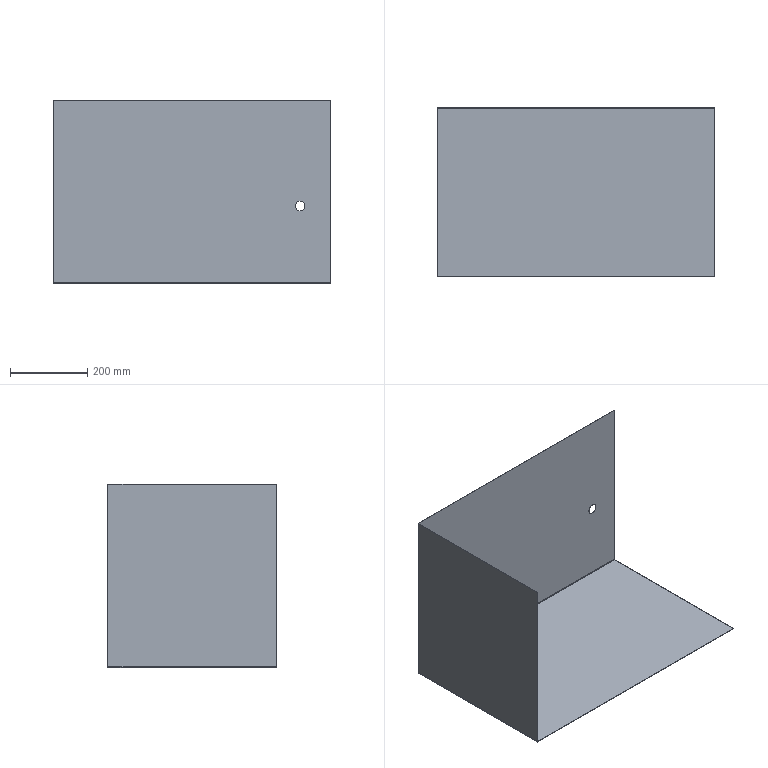Part | 1 solid | 24 faces | box 721 x 440 x 475 mm | volume 1037227 mm3 | plane 16 | cylinder 6 | spline 2 | commonest cylinder face diameters 1.473 x2 3.873 x2 25 x2
STEP:
#1=CARTESIAN_POINT('',(280.5,220.,212.5));
#2=VERTEX_POINT('',#1);
#3=CARTESIAN_POINT('',(280.5,220.,187.5));
#4=VERTEX_POINT('',#3);
#5=CARTESIAN_POINT('',(280.5,220.,200.));
#6=DIRECTION('',(0.,-1.,0.));
#7=DIRECTION('',(0.,0.,-1.));
#8=AXIS2_PLACEMENT_3D('',#5,#6,#7);
#9=CIRCLE('',#8,12.5);
#10=EDGE_CURVE('',#2,#4,#9,.T.);
#11=ORIENTED_EDGE('',*,*,#10,.F.);
#12=CARTESIAN_POINT('',(280.5,218.8,212.5));
#13=VERTEX_POINT('',#12);
#14=CARTESIAN_POINT('',(280.5,220.,212.5));
#15=DIRECTION('',(0.,-1.,0.));
#16=VECTOR('',#15,1000.);
#17=LINE('',#14,#16);
#18=EDGE_CURVE('',#2,#13,#17,.T.);
#19=ORIENTED_EDGE('',*,*,#18,.T.);
#20=CARTESIAN_POINT('',(280.5,218.8,187.5));
#21=VERTEX_POINT('',#20);
#22=CARTESIAN_POINT('',(280.5,218.8,200.));
#23=DIRECTION('',(0.,-1.,0.));
#24=DIRECTION('',(0.,0.,-1.));
#25=AXIS2_PLACEMENT_3D('',#22,#23,#24);
#26=CIRCLE('',#25,12.5);
#27=EDGE_CURVE('',#13,#21,#26,.T.);
#28=ORIENTED_EDGE('',*,*,#27,.T.);
#29=CARTESIAN_POINT('',(280.5,220.,187.5));
#30=DIRECTION('',(0.,-1.,0.));
#31=VECTOR('',#30,1000.);
#32=LINE('',#29,#31);
#33=EDGE_CURVE('',#4,#21,#32,.T.);
#34=ORIENTED_EDGE('',*,*,#33,.F.);
#35=EDGE_LOOP('',(#11,#19,#28,#34));
#36=FACE_OUTER_BOUND('',#35,.T.);
#37=CARTESIAN_POINT('',(280.5,220.,200.));
#38=DIRECTION('',(0.,-1.,0.));
#39=DIRECTION('',(0.,0.,-1.));
#40=AXIS2_PLACEMENT_3D('',#37,#38,#39);
#41=CYLINDRICAL_SURFACE('',#40,12.5);
#42=ADVANCED_FACE('',(#36),#41,.F.);
#43=CARTESIAN_POINT('',(-358.563,-220.,-1.2));
#44=VERTEX_POINT('',#43);
#45=CARTESIAN_POINT('',(-358.563,218.063,-1.2));
#46=VERTEX_POINT('',#45);
#47=CARTESIAN_POINT('',(-358.563,-220.,-1.2));
#48=DIRECTION('',(0.,1.,0.));
#49=VECTOR('',#48,1000.);
#50=LINE('',#47,#49);
#51=EDGE_CURVE('',#44,#46,#50,.T.);
#52=ORIENTED_EDGE('',*,*,#51,.T.);
#53=CARTESIAN_POINT('',(360.5,218.063,-1.2));
#54=VERTEX_POINT('',#53);
#55=CARTESIAN_POINT('',(-358.593,218.063,-1.2));
#56=DIRECTION('',(1.,0.,0.));
#57=VECTOR('',#56,1000.);
#58=LINE('',#55,#57);
#59=EDGE_CURVE('',#46,#54,#58,.T.);
#60=ORIENTED_EDGE('',*,*,#59,.T.);
#61=CARTESIAN_POINT('',(360.5,-220.,-1.2));
#62=VERTEX_POINT('',#61);
#63=CARTESIAN_POINT('',(360.5,220.,-1.2));
#64=DIRECTION('',(0.,1.,0.));
#65=VECTOR('',#64,1000.);
#66=LINE('',#63,#65);
#67=EDGE_CURVE('',#62,#54,#66,.T.);
#68=ORIENTED_EDGE('',*,*,#67,.F.);
#69=CARTESIAN_POINT('',(-360.5,-220.,-1.2));
#70=DIRECTION('',(1.,0.,0.));
#71=VECTOR('',#70,1000.);
#72=LINE('',#69,#71);
#73=EDGE_CURVE('',#44,#62,#72,.T.);
#74=ORIENTED_EDGE('',*,*,#73,.F.);
#75=EDGE_LOOP('',(#52,#60,#68,#74));
#76=FACE_OUTER_BOUND('',#75,.T.);
#77=CARTESIAN_POINT('',(0.,0.,-1.2));
#78=DIRECTION('',(0.,0.,1.));
#79=DIRECTION('',(1.,0.,0.));
#80=AXIS2_PLACEMENT_3D('',#77,#78,#79);
#81=PLANE('',#80);
#82=ADVANCED_FACE('',(#76),#81,.F.);
#83=CARTESIAN_POINT('',(-358.563,218.063,0.));
#84=VERTEX_POINT('',#83);
#85=CARTESIAN_POINT('',(360.5,218.063,0.));
#86=VERTEX_POINT('',#85);
#87=CARTESIAN_POINT('',(-358.593,218.063,0.));
#88=DIRECTION('',(1.,0.,0.));
#89=VECTOR('',#88,1000.);
#90=LINE('',#87,#89);
#91=EDGE_CURVE('',#84,#86,#90,.T.);
#92=ORIENTED_EDGE('',*,*,#91,.F.);
#93=CARTESIAN_POINT('',(-358.563,-220.,0.));
#94=VERTEX_POINT('',#93);
#95=CARTESIAN_POINT('',(-358.563,-220.,0.));
#96=DIRECTION('',(0.,1.,0.));
#97=VECTOR('',#96,1000.);
#98=LINE('',#95,#97);
#99=EDGE_CURVE('',#94,#84,#98,.T.);
#100=ORIENTED_EDGE('',*,*,#99,.F.);
#101=CARTESIAN_POINT('',(360.5,-220.,0.));
#102=VERTEX_POINT('',#101);
#103=CARTESIAN_POINT('',(-360.5,-220.,0.));
#104=DIRECTION('',(1.,0.,0.));
#105=VECTOR('',#104,1000.);
#106=LINE('',#103,#105);
#107=EDGE_CURVE('',#94,#102,#106,.T.);
#108=ORIENTED_EDGE('',*,*,#107,.T.);
#109=CARTESIAN_POINT('',(360.5,220.,0.));
#110=DIRECTION('',(0.,1.,0.));
#111=VECTOR('',#110,1000.);
#112=LINE('',#109,#111);
#113=EDGE_CURVE('',#102,#86,#112,.T.);
#114=ORIENTED_EDGE('',*,*,#113,.T.);
#115=EDGE_LOOP('',(#92,#100,#108,#114));
#116=FACE_OUTER_BOUND('',#115,.T.);
#117=CARTESIAN_POINT('',(0.,0.,0.));
#118=DIRECTION('',(0.,0.,1.));
#119=DIRECTION('',(1.,0.,0.));
#120=AXIS2_PLACEMENT_3D('',#117,#118,#119);
#121=PLANE('',#120);
#122=ADVANCED_FACE('',(#116),#121,.T.);
#123=ORIENTED_EDGE('',*,*,#107,.F.);
#124=CARTESIAN_POINT('',(-358.563,-220.,0.));
#125=DIRECTION('',(0.,0.,-1.));
#126=VECTOR('',#125,1000.);
#127=LINE('',#124,#126);
#128=EDGE_CURVE('',#94,#44,#127,.T.);
#129=ORIENTED_EDGE('',*,*,#128,.T.);
#130=ORIENTED_EDGE('',*,*,#73,.T.);
#131=CARTESIAN_POINT('',(360.5,-220.,-1.2));
#132=DIRECTION('',(0.,0.,1.));
#133=VECTOR('',#132,1000.);
#134=LINE('',#131,#133);
#135=EDGE_CURVE('',#62,#102,#134,.T.);
#136=ORIENTED_EDGE('',*,*,#135,.T.);
#137=EDGE_LOOP('',(#123,#129,#130,#136));
#138=FACE_OUTER_BOUND('',#137,.T.);
#139=CARTESIAN_POINT('',(-360.5,-220.,-1.2));
#140=DIRECTION('',(0.,-1.,0.));
#141=DIRECTION('',(0.,0.,-1.));
#142=AXIS2_PLACEMENT_3D('',#139,#140,#141);
#143=PLANE('',#142);
#144=ADVANCED_FACE('',(#138),#143,.T.);
#145=CARTESIAN_POINT('',(360.5,218.063,0.));
#146=DIRECTION('',(0.,0.,-1.));
#147=VECTOR('',#146,1000.);
#148=LINE('',#145,#147);
#149=EDGE_CURVE('',#86,#54,#148,.T.);
#150=ORIENTED_EDGE('',*,*,#149,.F.);
#151=ORIENTED_EDGE('',*,*,#113,.F.);
#152=ORIENTED_EDGE('',*,*,#135,.F.);
#153=ORIENTED_EDGE('',*,*,#67,.T.);
#154=EDGE_LOOP('',(#150,#151,#152,#153));
#155=FACE_OUTER_BOUND('',#154,.T.);
#156=CARTESIAN_POINT('',(360.5,220.,-1.2));
#157=DIRECTION('',(1.,0.,0.));
#158=DIRECTION('',(0.,1.,0.));
#159=AXIS2_PLACEMENT_3D('',#156,#157,#158);
#160=PLANE('',#159);
#161=ADVANCED_FACE('',(#155),#160,.T.);
#162=CARTESIAN_POINT('',(360.5,218.8,0.7366));
#163=VERTEX_POINT('',#162);
#164=CARTESIAN_POINT('',(360.5,220.,0.7366));
#165=VERTEX_POINT('',#164);
#166=CARTESIAN_POINT('',(360.5,220.,0.7366));
#167=DIRECTION('',(0.,1.,0.));
#168=VECTOR('',#167,1000.);
#169=LINE('',#166,#168);
#170=EDGE_CURVE('',#163,#165,#169,.T.);
#171=ORIENTED_EDGE('',*,*,#170,.F.);
#172=CARTESIAN_POINT('',(360.5,218.063,0.7366));
#173=DIRECTION('',(1.,0.,0.));
#174=DIRECTION('',(0.,0.,1.));
#175=AXIS2_PLACEMENT_3D('',#172,#173,#174);
#176=CIRCLE('',#175,0.7366);
#177=EDGE_CURVE('',#86,#163,#176,.T.);
#178=ORIENTED_EDGE('',*,*,#177,.F.);
#179=ORIENTED_EDGE('',*,*,#149,.T.);
#180=CARTESIAN_POINT('',(360.5,218.063,0.7366));
#181=DIRECTION('',(1.,0.,0.));
#182=DIRECTION('',(0.,0.,1.));
#183=AXIS2_PLACEMENT_3D('',#180,#181,#182);
#184=CIRCLE('',#183,1.937);
#185=EDGE_CURVE('',#54,#165,#184,.T.);
#186=ORIENTED_EDGE('',*,*,#185,.T.);
#187=EDGE_LOOP('',(#171,#178,#179,#186));
#188=FACE_OUTER_BOUND('',#187,.T.);
#189=CARTESIAN_POINT('',(360.5,218.063,0.7366));
#190=DIRECTION('',(1.,0.,0.));
#191=DIRECTION('',(0.,0.,-1.));
#192=AXIS2_PLACEMENT_3D('',#189,#190,#191);
#193=PLANE('',#192);
#194=ADVANCED_FACE('',(#188),#193,.T.);
#195=CARTESIAN_POINT('',(-358.593,218.8,0.7366));
#196=VERTEX_POINT('',#195);
#197=CARTESIAN_POINT('',(-358.593,218.8,0.7366));
#198=CARTESIAN_POINT('',(-358.588,218.8,0.5438));
#199=CARTESIAN_POINT('',(-358.583,218.721,0.3521));
#200=CARTESIAN_POINT('',(-358.573,218.448,0.07939));
#201=CARTESIAN_POINT('',(-358.568,218.256,0.));
#202=CARTESIAN_POINT('',(-358.563,218.063,0.));
#203=B_SPLINE_CURVE_WITH_KNOTS('',3,(#197,#198,#199,#200,#201,#202),.UNSPECIFIED.,.F.,.F.,(4,2,4),(0.,0.5,1.),.UNSPECIFIED.);
#204=EDGE_CURVE('',#196,#84,#203,.T.);
#205=ORIENTED_EDGE('',*,*,#204,.F.);
#206=CARTESIAN_POINT('',(-358.593,220.,0.7366));
#207=VERTEX_POINT('',#206);
#208=CARTESIAN_POINT('',(-358.593,218.8,0.7366));
#209=DIRECTION('',(0.,-1.,0.));
#210=VECTOR('',#209,1000.);
#211=LINE('',#208,#210);
#212=EDGE_CURVE('',#207,#196,#211,.T.);
#213=ORIENTED_EDGE('',*,*,#212,.F.);
#214=CARTESIAN_POINT('',(-358.593,220.,0.7366));
#215=CARTESIAN_POINT('',(-358.59,220.,0.4831));
#216=CARTESIAN_POINT('',(-358.588,219.95,0.2297));
#217=CARTESIAN_POINT('',(-358.583,219.756,-0.2387));
#218=CARTESIAN_POINT('',(-358.581,219.612,-0.4535));
#219=CARTESIAN_POINT('',(-358.576,219.254,-0.812));
#220=CARTESIAN_POINT('',(-358.573,219.039,-0.9556));
#221=CARTESIAN_POINT('',(-358.568,218.57,-1.15));
#222=CARTESIAN_POINT('',(-358.566,218.317,-1.2));
#223=CARTESIAN_POINT('',(-358.563,218.063,-1.2));
#224=B_SPLINE_CURVE_WITH_KNOTS('',3,(#214,#215,#216,#217,#218,#219,#220,#221,#222,#223),.UNSPECIFIED.,.F.,.F.,(4,2,2,2,4),(0.,0.25,0.5,0.75,1.),.UNSPECIFIED.);
#225=EDGE_CURVE('',#207,#46,#224,.T.);
#226=ORIENTED_EDGE('',*,*,#225,.T.);
#227=CARTESIAN_POINT('',(-358.563,218.063,0.));
#228=DIRECTION('',(0.,0.,-1.));
#229=VECTOR('',#228,1000.);
#230=LINE('',#227,#229);
#231=EDGE_CURVE('',#84,#46,#230,.T.);
#232=ORIENTED_EDGE('',*,*,#231,.F.);
#233=EDGE_LOOP('',(#205,#213,#226,#232));
#234=FACE_OUTER_BOUND('',#233,.T.);
#235=CARTESIAN_POINT('',(-358.593,220.012,0.7366));
#236=CARTESIAN_POINT('',(-358.59,220.012,0.4815));
#237=CARTESIAN_POINT('',(-358.588,219.961,0.2266));
#238=CARTESIAN_POINT('',(-358.583,219.766,-0.2448));
#239=CARTESIAN_POINT('',(-358.581,219.622,-0.4609));
#240=CARTESIAN_POINT('',(-358.576,219.261,-0.8216));
#241=CARTESIAN_POINT('',(-358.573,219.045,-0.9661));
#242=CARTESIAN_POINT('',(-358.568,218.573,-1.161));
#243=CARTESIAN_POINT('',(-358.566,218.319,-1.212));
#244=CARTESIAN_POINT('',(-358.563,218.063,-1.212));
#245=CARTESIAN_POINT('',(-358.593,220.,0.7366));
#246=CARTESIAN_POINT('',(-358.59,220.,0.4831));
#247=CARTESIAN_POINT('',(-358.588,219.95,0.2297));
#248=CARTESIAN_POINT('',(-358.583,219.756,-0.2387));
#249=CARTESIAN_POINT('',(-358.581,219.612,-0.4535));
#250=CARTESIAN_POINT('',(-358.576,219.254,-0.812));
#251=CARTESIAN_POINT('',(-358.573,219.039,-0.9556));
#252=CARTESIAN_POINT('',(-358.568,218.57,-1.15));
#253=CARTESIAN_POINT('',(-358.566,218.317,-1.2));
#254=CARTESIAN_POINT('',(-358.563,218.063,-1.2));
#255=CARTESIAN_POINT('',(-358.593,218.8,0.7366));
#256=CARTESIAN_POINT('',(-358.59,218.8,0.6402));
#257=CARTESIAN_POINT('',(-358.588,218.781,0.5438));
#258=CARTESIAN_POINT('',(-358.583,218.707,0.3656));
#259=CARTESIAN_POINT('',(-358.581,218.652,0.2839));
#260=CARTESIAN_POINT('',(-358.576,218.516,0.1476));
#261=CARTESIAN_POINT('',(-358.573,218.434,0.09297));
#262=CARTESIAN_POINT('',(-358.568,218.256,0.01917));
#263=CARTESIAN_POINT('',(-358.566,218.16,0.));
#264=CARTESIAN_POINT('',(-358.563,218.063,0.));
#265=CARTESIAN_POINT('',(-358.593,218.788,0.7366));
#266=CARTESIAN_POINT('',(-358.59,218.788,0.6417));
#267=CARTESIAN_POINT('',(-358.588,218.769,0.547));
#268=CARTESIAN_POINT('',(-358.583,218.696,0.3717));
#269=CARTESIAN_POINT('',(-358.581,218.643,0.2914));
#270=CARTESIAN_POINT('',(-358.576,218.509,0.1573));
#271=CARTESIAN_POINT('',(-358.573,218.428,0.1036));
#272=CARTESIAN_POINT('',(-358.568,218.253,0.03098));
#273=CARTESIAN_POINT('',(-358.566,218.158,0.01212));
#274=CARTESIAN_POINT('',(-358.563,218.063,0.01212));
#275=B_SPLINE_SURFACE_WITH_KNOTS('',1,3,((#235,#236,#237,#238,#239,#240,#241,#242,#243,#244),(#245,#246,#247,#248,#249,#250,#251,#252,#253,#254),(#255,#256,#257,#258,#259,#260,#261,#262,#263,#264),(#265,#266,#267,#268,#269,#270,#271,#272,#273,#274)),.UNSPECIFIED.,.F.,.F.,.F.,(2,1,1,2),(4,2,2,2,4),(-0.01,0.,1.,1.01),(0.,0.25,0.5,0.75,1.),.UNSPECIFIED.);
#276=ADVANCED_FACE('',(#234),#275,.F.);
#277=ORIENTED_EDGE('',*,*,#59,.F.);
#278=ORIENTED_EDGE('',*,*,#225,.F.);
#279=CARTESIAN_POINT('',(0.,220.,0.7366));
#280=DIRECTION('',(-1.,0.,0.));
#281=VECTOR('',#280,1000.);
#282=LINE('',#279,#281);
#283=EDGE_CURVE('',#165,#207,#282,.T.);
#284=ORIENTED_EDGE('',*,*,#283,.F.);
#285=ORIENTED_EDGE('',*,*,#185,.F.);
#286=EDGE_LOOP('',(#277,#278,#284,#285));
#287=FACE_OUTER_BOUND('',#286,.T.);
#288=CARTESIAN_POINT('',(-358.593,218.063,0.7366));
#289=DIRECTION('',(-1.,0.,0.));
#290=DIRECTION('',(0.,1.,0.));
#291=AXIS2_PLACEMENT_3D('',#288,#289,#290);
#292=CYLINDRICAL_SURFACE('',#291,1.937);
#293=ADVANCED_FACE('',(#287),#292,.T.);
#294=ORIENTED_EDGE('',*,*,#91,.T.);
#295=ORIENTED_EDGE('',*,*,#177,.T.);
#296=CARTESIAN_POINT('',(360.5,218.8,0.7366));
#297=DIRECTION('',(-1.,0.,0.));
#298=VECTOR('',#297,1000.);
#299=LINE('',#296,#298);
#300=EDGE_CURVE('',#163,#196,#299,.T.);
#301=ORIENTED_EDGE('',*,*,#300,.T.);
#302=ORIENTED_EDGE('',*,*,#204,.T.);
#303=EDGE_LOOP('',(#294,#295,#301,#302));
#304=FACE_OUTER_BOUND('',#303,.T.);
#305=CARTESIAN_POINT('',(-358.593,218.063,0.7366));
#306=DIRECTION('',(-1.,0.,0.));
#307=DIRECTION('',(0.,1.,0.));
#308=AXIS2_PLACEMENT_3D('',#305,#306,#307);
#309=CYLINDRICAL_SURFACE('',#308,0.7366);
#310=ADVANCED_FACE('',(#304),#309,.F.);
#311=CARTESIAN_POINT('',(360.5,218.8,473.8));
#312=VERTEX_POINT('',#311);
#313=CARTESIAN_POINT('',(360.5,218.8,0.));
#314=DIRECTION('',(0.,0.,1.));
#315=VECTOR('',#314,1000.);
#316=LINE('',#313,#315);
#317=EDGE_CURVE('',#163,#312,#316,.T.);
#318=ORIENTED_EDGE('',*,*,#317,.F.);
#319=ORIENTED_EDGE('',*,*,#170,.T.);
#320=CARTESIAN_POINT('',(360.5,220.,473.8));
#321=VERTEX_POINT('',#320);
#322=CARTESIAN_POINT('',(360.5,220.,473.8));
#323=DIRECTION('',(0.,0.,1.));
#324=VECTOR('',#323,1000.);
#325=LINE('',#322,#324);
#326=EDGE_CURVE('',#165,#321,#325,.T.);
#327=ORIENTED_EDGE('',*,*,#326,.T.);
#328=CARTESIAN_POINT('',(360.5,220.,473.8));
#329=DIRECTION('',(0.,-1.,0.));
#330=VECTOR('',#329,1000.);
#331=LINE('',#328,#330);
#332=EDGE_CURVE('',#321,#312,#331,.T.);
#333=ORIENTED_EDGE('',*,*,#332,.T.);
#334=EDGE_LOOP('',(#318,#319,#327,#333));
#335=FACE_OUTER_BOUND('',#334,.T.);
#336=CARTESIAN_POINT('',(360.5,220.,473.8));
#337=DIRECTION('',(1.,0.,0.));
#338=DIRECTION('',(0.,0.,-1.));
#339=AXIS2_PLACEMENT_3D('',#336,#337,#338);
#340=PLANE('',#339);
#341=ADVANCED_FACE('',(#335),#340,.T.);
#342=CARTESIAN_POINT('',(280.5,220.,200.));
#343=DIRECTION('',(0.,-1.,0.));
#344=DIRECTION('',(0.,0.,-1.));
#345=AXIS2_PLACEMENT_3D('',#342,#343,#344);
#346=CIRCLE('',#345,12.5);
#347=EDGE_CURVE('',#4,#2,#346,.T.);
#348=ORIENTED_EDGE('',*,*,#347,.T.);
#349=ORIENTED_EDGE('',*,*,#10,.T.);
#350=EDGE_LOOP('',(#348,#349));
#351=FACE_BOUND('',#350,.T.);
#352=CARTESIAN_POINT('',(-358.593,220.,473.8));
#353=VERTEX_POINT('',#352);
#354=CARTESIAN_POINT('',(-358.593,220.,0.));
#355=DIRECTION('',(0.,0.,-1.));
#356=VECTOR('',#355,1000.);
#357=LINE('',#354,#356);
#358=EDGE_CURVE('',#353,#207,#357,.T.);
#359=ORIENTED_EDGE('',*,*,#358,.F.);
#360=CARTESIAN_POINT('',(-360.5,220.,473.8));
#361=DIRECTION('',(-1.,0.,0.));
#362=VECTOR('',#361,1000.);
#363=LINE('',#360,#362);
#364=EDGE_CURVE('',#321,#353,#363,.T.);
#365=ORIENTED_EDGE('',*,*,#364,.F.);
#366=ORIENTED_EDGE('',*,*,#326,.F.);
#367=ORIENTED_EDGE('',*,*,#283,.T.);
#368=EDGE_LOOP('',(#359,#365,#366,#367));
#369=FACE_OUTER_BOUND('',#368,.T.);
#370=CARTESIAN_POINT('',(0.,220.,0.));
#371=DIRECTION('',(0.,1.,0.));
#372=DIRECTION('',(0.,0.,1.));
#373=AXIS2_PLACEMENT_3D('',#370,#371,#372);
#374=PLANE('',#373);
#375=ADVANCED_FACE('',(#351,#369),#374,.T.);
#376=CARTESIAN_POINT('',(280.5,218.8,200.));
#377=DIRECTION('',(0.,-1.,0.));
#378=DIRECTION('',(0.,0.,-1.));
#379=AXIS2_PLACEMENT_3D('',#376,#377,#378);
#380=CIRCLE('',#379,12.5);
#381=EDGE_CURVE('',#21,#13,#380,.T.);
#382=ORIENTED_EDGE('',*,*,#381,.F.);
#383=ORIENTED_EDGE('',*,*,#27,.F.);
#384=EDGE_LOOP('',(#382,#383));
#385=FACE_BOUND('',#384,.T.);
#386=CARTESIAN_POINT('',(-358.593,218.8,473.8));
#387=VERTEX_POINT('',#386);
#388=CARTESIAN_POINT('',(0.,218.8,473.8));
#389=DIRECTION('',(-1.,0.,0.));
#390=VECTOR('',#389,1000.);
#391=LINE('',#388,#390);
#392=EDGE_CURVE('',#312,#387,#391,.T.);
#393=ORIENTED_EDGE('',*,*,#392,.T.);
#394=CARTESIAN_POINT('',(-358.593,218.8,0.));
#395=DIRECTION('',(0.,0.,1.));
#396=VECTOR('',#395,1000.);
#397=LINE('',#394,#396);
#398=EDGE_CURVE('',#196,#387,#397,.T.);
#399=ORIENTED_EDGE('',*,*,#398,.F.);
#400=ORIENTED_EDGE('',*,*,#300,.F.);
#401=ORIENTED_EDGE('',*,*,#317,.T.);
#402=EDGE_LOOP('',(#393,#399,#400,#401));
#403=FACE_OUTER_BOUND('',#402,.T.);
#404=CARTESIAN_POINT('',(0.,218.8,0.));
#405=DIRECTION('',(0.,1.,0.));
#406=DIRECTION('',(0.,0.,1.));
#407=AXIS2_PLACEMENT_3D('',#404,#405,#406);
#408=PLANE('',#407);
#409=ADVANCED_FACE('',(#385,#403),#408,.F.);
#410=CARTESIAN_POINT('',(-358.593,218.8,473.8));
#411=DIRECTION('',(0.,1.,0.));
#412=VECTOR('',#411,1000.);
#413=LINE('',#410,#412);
#414=EDGE_CURVE('',#387,#353,#413,.T.);
#415=ORIENTED_EDGE('',*,*,#414,.F.);
#416=ORIENTED_EDGE('',*,*,#392,.F.);
#417=ORIENTED_EDGE('',*,*,#332,.F.);
#418=ORIENTED_EDGE('',*,*,#364,.T.);
#419=EDGE_LOOP('',(#415,#416,#417,#418));
#420=FACE_OUTER_BOUND('',#419,.T.);
#421=CARTESIAN_POINT('',(-360.5,220.,473.8));
#422=DIRECTION('',(0.,0.,1.));
#423=DIRECTION('',(0.,-1.,0.));
#424=AXIS2_PLACEMENT_3D('',#421,#422,#423);
#425=PLANE('',#424);
#426=ADVANCED_FACE('',(#420),#425,.T.);
#427=ORIENTED_EDGE('',*,*,#398,.T.);
#428=ORIENTED_EDGE('',*,*,#414,.T.);
#429=ORIENTED_EDGE('',*,*,#358,.T.);
#430=ORIENTED_EDGE('',*,*,#212,.T.);
#431=EDGE_LOOP('',(#427,#428,#429,#430));
#432=FACE_OUTER_BOUND('',#431,.T.);
#433=CARTESIAN_POINT('',(-358.593,218.8,0.));
#434=DIRECTION('',(1.,0.,0.));
#435=DIRECTION('',(0.,0.,-1.));
#436=AXIS2_PLACEMENT_3D('',#433,#434,#435);
#437=PLANE('',#436);
#438=ADVANCED_FACE('',(#432),#437,.F.);
#439=CARTESIAN_POINT('',(-360.5,218.093,0.7366));
#440=VERTEX_POINT('',#439);
#441=CARTESIAN_POINT('',(-359.3,218.093,0.7366));
#442=VERTEX_POINT('',#441);
#443=CARTESIAN_POINT('',(-359.3,218.093,0.7366));
#444=DIRECTION('',(1.,0.,0.));
#445=VECTOR('',#444,1000.);
#446=LINE('',#443,#445);
#447=EDGE_CURVE('',#440,#442,#446,.T.);
#448=ORIENTED_EDGE('',*,*,#447,.T.);
#449=CARTESIAN_POINT('',(-358.563,218.063,0.));
#450=CARTESIAN_POINT('',(-358.756,218.068,0.));
#451=CARTESIAN_POINT('',(-358.948,218.073,0.07939));
#452=CARTESIAN_POINT('',(-359.221,218.083,0.3521));
#453=CARTESIAN_POINT('',(-359.3,218.088,0.5438));
#454=CARTESIAN_POINT('',(-359.3,218.093,0.7366));
#455=B_SPLINE_CURVE_WITH_KNOTS('',3,(#449,#450,#451,#452,#453,#454),.UNSPECIFIED.,.F.,.F.,(4,2,4),(0.,0.5,1.),.UNSPECIFIED.);
#456=EDGE_CURVE('',#84,#442,#455,.T.);
#457=ORIENTED_EDGE('',*,*,#456,.F.);
#458=ORIENTED_EDGE('',*,*,#231,.T.);
#459=CARTESIAN_POINT('',(-358.563,218.063,-1.2));
#460=CARTESIAN_POINT('',(-358.817,218.066,-1.2));
#461=CARTESIAN_POINT('',(-359.07,218.068,-1.15));
#462=CARTESIAN_POINT('',(-359.539,218.073,-0.9556));
#463=CARTESIAN_POINT('',(-359.754,218.076,-0.812));
#464=CARTESIAN_POINT('',(-360.112,218.081,-0.4535));
#465=CARTESIAN_POINT('',(-360.256,218.083,-0.2387));
#466=CARTESIAN_POINT('',(-360.45,218.088,0.2297));
#467=CARTESIAN_POINT('',(-360.5,218.09,0.4831));
#468=CARTESIAN_POINT('',(-360.5,218.093,0.7366));
#469=B_SPLINE_CURVE_WITH_KNOTS('',3,(#459,#460,#461,#462,#463,#464,#465,#466,#467,#468),.UNSPECIFIED.,.F.,.F.,(4,2,2,2,4),(0.,0.25,0.5,0.75,1.),.UNSPECIFIED.);
#470=EDGE_CURVE('',#46,#440,#469,.T.);
#471=ORIENTED_EDGE('',*,*,#470,.T.);
#472=EDGE_LOOP('',(#448,#457,#458,#471));
#473=FACE_OUTER_BOUND('',#472,.T.);
#474=CARTESIAN_POINT('',(-358.563,218.063,-1.212));
#475=CARTESIAN_POINT('',(-358.819,218.066,-1.212));
#476=CARTESIAN_POINT('',(-359.073,218.068,-1.161));
#477=CARTESIAN_POINT('',(-359.545,218.073,-0.9661));
#478=CARTESIAN_POINT('',(-359.761,218.076,-0.8216));
#479=CARTESIAN_POINT('',(-360.122,218.081,-0.4609));
#480=CARTESIAN_POINT('',(-360.266,218.083,-0.2448));
#481=CARTESIAN_POINT('',(-360.461,218.088,0.2266));
#482=CARTESIAN_POINT('',(-360.512,218.09,0.4815));
#483=CARTESIAN_POINT('',(-360.512,218.093,0.7366));
#484=CARTESIAN_POINT('',(-358.563,218.063,-1.2));
#485=CARTESIAN_POINT('',(-358.817,218.066,-1.2));
#486=CARTESIAN_POINT('',(-359.07,218.068,-1.15));
#487=CARTESIAN_POINT('',(-359.539,218.073,-0.9556));
#488=CARTESIAN_POINT('',(-359.754,218.076,-0.812));
#489=CARTESIAN_POINT('',(-360.112,218.081,-0.4535));
#490=CARTESIAN_POINT('',(-360.256,218.083,-0.2387));
#491=CARTESIAN_POINT('',(-360.45,218.088,0.2297));
#492=CARTESIAN_POINT('',(-360.5,218.09,0.4831));
#493=CARTESIAN_POINT('',(-360.5,218.093,0.7366));
#494=CARTESIAN_POINT('',(-358.563,218.063,0.));
#495=CARTESIAN_POINT('',(-358.66,218.066,0.));
#496=CARTESIAN_POINT('',(-358.756,218.068,0.01917));
#497=CARTESIAN_POINT('',(-358.934,218.073,0.09297));
#498=CARTESIAN_POINT('',(-359.016,218.076,0.1476));
#499=CARTESIAN_POINT('',(-359.152,218.081,0.2839));
#500=CARTESIAN_POINT('',(-359.207,218.083,0.3656));
#501=CARTESIAN_POINT('',(-359.281,218.088,0.5438));
#502=CARTESIAN_POINT('',(-359.3,218.09,0.6402));
#503=CARTESIAN_POINT('',(-359.3,218.093,0.7366));
#504=CARTESIAN_POINT('',(-358.563,218.063,0.01212));
#505=CARTESIAN_POINT('',(-358.658,218.066,0.01212));
#506=CARTESIAN_POINT('',(-358.753,218.068,0.03098));
#507=CARTESIAN_POINT('',(-358.928,218.073,0.1036));
#508=CARTESIAN_POINT('',(-359.009,218.076,0.1573));
#509=CARTESIAN_POINT('',(-359.143,218.081,0.2914));
#510=CARTESIAN_POINT('',(-359.196,218.083,0.3717));
#511=CARTESIAN_POINT('',(-359.269,218.088,0.547));
#512=CARTESIAN_POINT('',(-359.288,218.09,0.6417));
#513=CARTESIAN_POINT('',(-359.288,218.093,0.7366));
#514=B_SPLINE_SURFACE_WITH_KNOTS('',1,3,((#474,#475,#476,#477,#478,#479,#480,#481,#482,#483),(#484,#485,#486,#487,#488,#489,#490,#491,#492,#493),(#494,#495,#496,#497,#498,#499,#500,#501,#502,#503),(#504,#505,#506,#507,#508,#509,#510,#511,#512,#513)),.UNSPECIFIED.,.F.,.F.,.F.,(2,1,1,2),(4,2,2,2,4),(-0.01,0.,1.,1.01),(0.,0.25,0.5,0.75,1.),.UNSPECIFIED.);
#515=ADVANCED_FACE('',(#473),#514,.F.);
#516=CARTESIAN_POINT('',(-359.3,-220.,0.7366));
#517=VERTEX_POINT('',#516);
#518=CARTESIAN_POINT('',(-358.563,-220.,0.7366));
#519=DIRECTION('',(0.,-1.,0.));
#520=DIRECTION('',(0.,0.,-1.));
#521=AXIS2_PLACEMENT_3D('',#518,#519,#520);
#522=CIRCLE('',#521,0.7366);
#523=EDGE_CURVE('',#517,#94,#522,.T.);
#524=ORIENTED_EDGE('',*,*,#523,.F.);
#525=CARTESIAN_POINT('',(-360.5,-220.,0.7366));
#526=VERTEX_POINT('',#525);
#527=CARTESIAN_POINT('',(-359.3,-220.,0.7366));
#528=DIRECTION('',(-1.,0.,0.));
#529=VECTOR('',#528,1000.);
#530=LINE('',#527,#529);
#531=EDGE_CURVE('',#517,#526,#530,.T.);
#532=ORIENTED_EDGE('',*,*,#531,.T.);
#533=CARTESIAN_POINT('',(-358.563,-220.,0.7366));
#534=DIRECTION('',(0.,-1.,0.));
#535=DIRECTION('',(0.,0.,-1.));
#536=AXIS2_PLACEMENT_3D('',#533,#534,#535);
#537=CIRCLE('',#536,1.937);
#538=EDGE_CURVE('',#526,#44,#537,.T.);
#539=ORIENTED_EDGE('',*,*,#538,.T.);
#540=ORIENTED_EDGE('',*,*,#128,.F.);
#541=EDGE_LOOP('',(#524,#532,#539,#540));
#542=FACE_OUTER_BOUND('',#541,.T.);
#543=CARTESIAN_POINT('',(-358.563,-220.,0.7366));
#544=DIRECTION('',(0.,1.,0.));
#545=DIRECTION('',(0.,0.,1.));
#546=AXIS2_PLACEMENT_3D('',#543,#544,#545);
#547=PLANE('',#546);
#548=ADVANCED_FACE('',(#542),#547,.F.);
#549=ORIENTED_EDGE('',*,*,#51,.F.);
#550=ORIENTED_EDGE('',*,*,#538,.F.);
#551=CARTESIAN_POINT('',(-360.5,220.,0.7366));
#552=DIRECTION('',(0.,1.,0.));
#553=VECTOR('',#552,1000.);
#554=LINE('',#551,#553);
#555=EDGE_CURVE('',#526,#440,#554,.T.);
#556=ORIENTED_EDGE('',*,*,#555,.T.);
#557=ORIENTED_EDGE('',*,*,#470,.F.);
#558=EDGE_LOOP('',(#549,#550,#556,#557));
#559=FACE_OUTER_BOUND('',#558,.T.);
#560=CARTESIAN_POINT('',(-358.563,-220.,0.7366));
#561=DIRECTION('',(0.,-1.,0.));
#562=DIRECTION('',(-1.,0.,0.));
#563=AXIS2_PLACEMENT_3D('',#560,#561,#562);
#564=CYLINDRICAL_SURFACE('',#563,1.937);
#565=ADVANCED_FACE('',(#559),#564,.T.);
#566=ORIENTED_EDGE('',*,*,#99,.T.);
#567=ORIENTED_EDGE('',*,*,#456,.T.);
#568=CARTESIAN_POINT('',(-359.3,220.,0.7366));
#569=DIRECTION('',(0.,-1.,0.));
#570=VECTOR('',#569,1000.);
#571=LINE('',#568,#570);
#572=EDGE_CURVE('',#442,#517,#571,.T.);
#573=ORIENTED_EDGE('',*,*,#572,.T.);
#574=ORIENTED_EDGE('',*,*,#523,.T.);
#575=EDGE_LOOP('',(#566,#567,#573,#574));
#576=FACE_OUTER_BOUND('',#575,.T.);
#577=CARTESIAN_POINT('',(-358.563,-220.,0.7366));
#578=DIRECTION('',(0.,-1.,0.));
#579=DIRECTION('',(-1.,0.,0.));
#580=AXIS2_PLACEMENT_3D('',#577,#578,#579);
#581=CYLINDRICAL_SURFACE('',#580,0.7366);
#582=ADVANCED_FACE('',(#576),#581,.F.);
#583=CARTESIAN_POINT('',(-359.3,218.093,473.8));
#584=VERTEX_POINT('',#583);
#585=CARTESIAN_POINT('',(-360.5,218.093,473.8));
#586=VERTEX_POINT('',#585);
#587=CARTESIAN_POINT('',(-360.5,218.093,473.8));
#588=DIRECTION('',(-1.,0.,0.));
#589=VECTOR('',#588,1000.);
#590=LINE('',#587,#589);
#591=EDGE_CURVE('',#584,#586,#590,.T.);
#592=ORIENTED_EDGE('',*,*,#591,.F.);
#593=CARTESIAN_POINT('',(-359.3,218.093,0.));
#594=DIRECTION('',(0.,0.,1.));
#595=VECTOR('',#594,1000.);
#596=LINE('',#593,#595);
#597=EDGE_CURVE('',#442,#584,#596,.T.);
#598=ORIENTED_EDGE('',*,*,#597,.F.);
#599=ORIENTED_EDGE('',*,*,#447,.F.);
#600=CARTESIAN_POINT('',(-360.5,218.093,0.));
#601=DIRECTION('',(0.,0.,1.));
#602=VECTOR('',#601,1000.);
#603=LINE('',#600,#602);
#604=EDGE_CURVE('',#440,#586,#603,.T.);
#605=ORIENTED_EDGE('',*,*,#604,.T.);
#606=EDGE_LOOP('',(#592,#598,#599,#605));
#607=FACE_OUTER_BOUND('',#606,.T.);
#608=CARTESIAN_POINT('',(-359.3,218.093,0.));
#609=DIRECTION('',(0.,1.,0.));
#610=DIRECTION('',(0.,0.,1.));
#611=AXIS2_PLACEMENT_3D('',#608,#609,#610);
#612=PLANE('',#611);
#613=ADVANCED_FACE('',(#607),#612,.T.);
#614=ORIENTED_EDGE('',*,*,#604,.F.);
#615=ORIENTED_EDGE('',*,*,#555,.F.);
#616=CARTESIAN_POINT('',(-360.5,-220.,473.8));
#617=VERTEX_POINT('',#616);
#618=CARTESIAN_POINT('',(-360.5,-220.,473.8));
#619=DIRECTION('',(0.,0.,-1.));
#620=VECTOR('',#619,1000.);
#621=LINE('',#618,#620);
#622=EDGE_CURVE('',#617,#526,#621,.T.);
#623=ORIENTED_EDGE('',*,*,#622,.F.);
#624=CARTESIAN_POINT('',(-360.5,220.,473.8));
#625=DIRECTION('',(0.,-1.,0.));
#626=VECTOR('',#625,1000.);
#627=LINE('',#624,#626);
#628=EDGE_CURVE('',#586,#617,#627,.T.);
#629=ORIENTED_EDGE('',*,*,#628,.F.);
#630=EDGE_LOOP('',(#614,#615,#623,#629));
#631=FACE_OUTER_BOUND('',#630,.T.);
#632=CARTESIAN_POINT('',(-360.5,0.,0.));
#633=DIRECTION('',(1.,0.,0.));
#634=DIRECTION('',(0.,0.,-1.));
#635=AXIS2_PLACEMENT_3D('',#632,#633,#634);
#636=PLANE('',#635);
#637=ADVANCED_FACE('',(#631),#636,.F.);
#638=ORIENTED_EDGE('',*,*,#572,.F.);
#639=ORIENTED_EDGE('',*,*,#597,.T.);
#640=CARTESIAN_POINT('',(-359.3,-220.,473.8));
#641=VERTEX_POINT('',#640);
#642=CARTESIAN_POINT('',(-359.3,0.,473.8));
#643=DIRECTION('',(0.,-1.,0.));
#644=VECTOR('',#643,1000.);
#645=LINE('',#642,#644);
#646=EDGE_CURVE('',#584,#641,#645,.T.);
#647=ORIENTED_EDGE('',*,*,#646,.T.);
#648=CARTESIAN_POINT('',(-359.3,-220.,0.));
#649=DIRECTION('',(0.,0.,-1.));
#650=VECTOR('',#649,1000.);
#651=LINE('',#648,#650);
#652=EDGE_CURVE('',#641,#517,#651,.T.);
#653=ORIENTED_EDGE('',*,*,#652,.T.);
#654=EDGE_LOOP('',(#638,#639,#647,#653));
#655=FACE_OUTER_BOUND('',#654,.T.);
#656=CARTESIAN_POINT('',(-359.3,0.,0.));
#657=DIRECTION('',(1.,0.,0.));
#658=DIRECTION('',(0.,0.,-1.));
#659=AXIS2_PLACEMENT_3D('',#656,#657,#658);
#660=PLANE('',#659);
#661=ADVANCED_FACE('',(#655),#660,.T.);
#662=ORIENTED_EDGE('',*,*,#646,.F.);
#663=ORIENTED_EDGE('',*,*,#591,.T.);
#664=ORIENTED_EDGE('',*,*,#628,.T.);
#665=CARTESIAN_POINT('',(-360.5,-220.,473.8));
#666=DIRECTION('',(1.,0.,0.));
#667=VECTOR('',#666,1000.);
#668=LINE('',#665,#667);
#669=EDGE_CURVE('',#617,#641,#668,.T.);
#670=ORIENTED_EDGE('',*,*,#669,.T.);
#671=EDGE_LOOP('',(#662,#663,#664,#670));
#672=FACE_OUTER_BOUND('',#671,.T.);
#673=CARTESIAN_POINT('',(-360.5,220.,473.8));
#674=DIRECTION('',(0.,0.,1.));
#675=DIRECTION('',(1.,0.,0.));
#676=AXIS2_PLACEMENT_3D('',#673,#674,#675);
#677=PLANE('',#676);
#678=ADVANCED_FACE('',(#672),#677,.T.);
#679=ORIENTED_EDGE('',*,*,#622,.T.);
#680=ORIENTED_EDGE('',*,*,#531,.F.);
#681=ORIENTED_EDGE('',*,*,#652,.F.);
#682=ORIENTED_EDGE('',*,*,#669,.F.);
#683=EDGE_LOOP('',(#679,#680,#681,#682));
#684=FACE_OUTER_BOUND('',#683,.T.);
#685=CARTESIAN_POINT('',(-360.5,-220.,473.8));
#686=DIRECTION('',(0.,-1.,0.));
#687=DIRECTION('',(0.,0.,-1.));
#688=AXIS2_PLACEMENT_3D('',#685,#686,#687);
#689=PLANE('',#688);
#690=ADVANCED_FACE('',(#684),#689,.T.);
#691=ORIENTED_EDGE('',*,*,#18,.F.);
#692=ORIENTED_EDGE('',*,*,#347,.F.);
#693=ORIENTED_EDGE('',*,*,#33,.T.);
#694=ORIENTED_EDGE('',*,*,#381,.T.);
#695=EDGE_LOOP('',(#691,#692,#693,#694));
#696=FACE_OUTER_BOUND('',#695,.T.);
#697=CARTESIAN_POINT('',(280.5,220.,200.));
#698=DIRECTION('',(0.,-1.,0.));
#699=DIRECTION('',(0.,0.,-1.));
#700=AXIS2_PLACEMENT_3D('',#697,#698,#699);
#701=CYLINDRICAL_SURFACE('',#700,12.5);
#702=ADVANCED_FACE('',(#696),#701,.F.);
#703=CLOSED_SHELL('',(#42,#82,#122,#144,#161,#194,#276,#293,#310,#341,#375,#409,#426,#438,#515,#548,#565,#582,#613,#637,#661,#678,#690,#702));
#704=MANIFOLD_SOLID_BREP('',#703);
#705=CARTESIAN_POINT('',(0.,0.,0.));
#706=DIRECTION('',(0.,0.,1.));
#707=DIRECTION('',(1.,0.,0.));
#708=AXIS2_PLACEMENT_3D('',#705,#706,#707);
#709=(LENGTH_UNIT()NAMED_UNIT(*)SI_UNIT(.MILLI.,.METRE.));
#710=UNCERTAINTY_MEASURE_WITH_UNIT(LENGTH_MEASURE(0.00001),#709,'','');
#711=(NAMED_UNIT(*)PLANE_ANGLE_UNIT()SI_UNIT($,.RADIAN.));
#712=(NAMED_UNIT(*)SI_UNIT($,.STERADIAN.)SOLID_ANGLE_UNIT());
#713=(GEOMETRIC_REPRESENTATION_CONTEXT(3)GLOBAL_UNCERTAINTY_ASSIGNED_CONTEXT((#710))GLOBAL_UNIT_ASSIGNED_CONTEXT((#709,#711,#712))REPRESENTATION_CONTEXT('',''));
#714=ADVANCED_BREP_SHAPE_REPRESENTATION('',(#704,#708),#713);